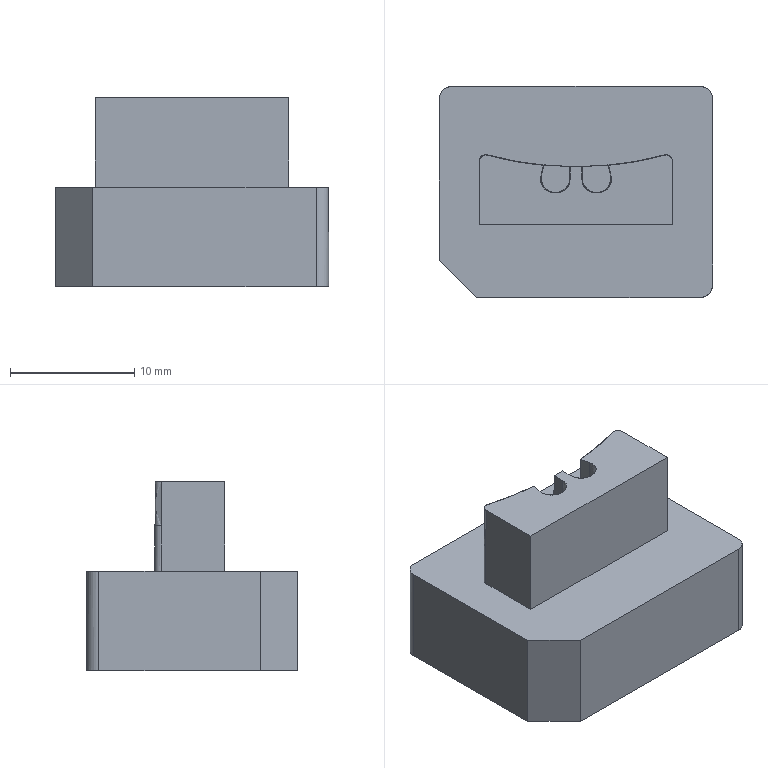NC program | PowerMill | posted by the shop | part box 22 x 17 x 15.232 mm
Lines 5583 to 7135 of 87032:
( TOOL ID   D1C_1_1 )
( TOOL DIA. 1. TIP RAD 0 LENGTH 58.8 )
( Z = -3.721 )
T27 M6
T3
G91 G28 Z0
G0 G90 G54
M08
S22000 M3
X0 Y0 M8
G43 Z9.812 H27
X-2.541 Y2.768
Z.962
G1 Z-.238 F1200
X-2.545 Y2.755 F2000
G3 X-2.454 Y2.605 I.12 J-.03
G1 X-2.412 Y2.594
X-2.315 Y2.533
X-2.171 Y2.359
X-2.144 Y2.292
X-2.123 Y2.051
X-2.29 Y1.327
X-2.323 Y1.086
X-2.299 Y.856
X-2.292 Y.835
X-2.171 Y.636
X-1.995 Y.507
X-1.976 Y.498
X-1.689 Y.44
X-1.447 Y.455
X-1.288 Y.519
X-1.09 Y.713
X-1.027 Y.844
X-.988 Y1.086
X-.99 Y1.915
X-1.45 Y1.92
X-1.459 Y1.085
G2 X-1.607 Y.923 I-.165 J.002
G1 X-1.675 Y.916
G2 X-1.846 Y1.064 I-.016 J.154
G1 X-1.849 Y1.137
X-1.847 Y1.162
X-1.674 Y1.943
X-1.643 Y1.992
X-1.587 Y2.008
X-1.53 Y2.005
X-1.473 Y1.979
X-1.45 Y1.92
X-.99 Y1.915
Y2.051
X-.965 Y2.177
X-.91 Y2.292
X-.724 Y2.458
X-.605 Y2.488
X-2.541 Y2.768 Z-.288
X-2.544 Y2.755
G3 X-2.454 Y2.605 I.12 J-.03
G1 X-2.412 Y2.595
X-2.31 Y2.533
X-2.171 Y2.363
X-2.143 Y2.292
X-2.122 Y2.051
X-2.322 Y1.086
X-2.299 Y.856
X-2.292 Y.834
X-2.171 Y.641
X-1.995 Y.507
X-1.981 Y.501
X-1.976 Y.499
X-1.97 Y.497
X-1.967
X-1.689 Y.441
X-1.447 Y.456
X-1.288 Y.519
X-1.272 Y.535
X-1.091 Y.713
X-1.028 Y.844
X-1.013 Y.929
X-1.007 Y.967
X-.995 Y1.808
X-1.457 Y1.823
X-1.479 Y1.138
G2 X-1.673 Y.971 I-.174 J.006
X-1.824 Y1.178 I.02 J.173
G1 X-1.672 Y1.943
X-1.642 Y1.992
X-1.586 Y2.009
X-1.532 Y2.006
X-1.476 Y1.979
X-1.454 Y1.921
X-1.457 Y1.823
X-.995 Y1.808
X-.991 Y2.051
X-.965 Y2.184
X-.911 Y2.292
X-.724 Y2.459
X-.607 Y2.488
X-2.54 Y2.769 Z-.337
X-2.544 Y2.755
G3 X-2.453 Y2.606 I.12 J-.03
G1 X-2.412 Y2.596
X-2.308 Y2.533
X-2.171 Y2.364
X-2.142 Y2.292
X-2.121 Y2.051
X-2.205 Y1.647
X-1.753 Y1.553
X-1.671 Y1.944
X-1.641 Y1.993
X-1.586 Y2.01
X-1.533 Y2.007
X-1.477 Y1.98
X-1.455 Y1.922
X-1.48 Y1.137
X-1.49 Y1.083
X-1.518 Y1.035
X-1.573 Y.965
G2 X-1.819 Y1.027 I-.109 J.087
G1 X-1.835 Y1.106
X-1.837 Y1.134
X-1.834 Y1.161
X-1.753 Y1.553
X-2.205 Y1.647
X-2.321 Y1.086
X-2.299 Y.856
X-2.292 Y.834
X-2.171 Y.642
X-2.164 Y.635
X-1.999 Y.511
X-1.995 Y.507
X-1.989 Y.505
X-1.972 Y.498
X-1.967 Y.497
X-1.701 Y.443
X-1.689 Y.441
X-1.447 Y.457
X-1.297 Y.516
X-1.283 Y.525
X-1.267 Y.541
X-1.092 Y.713
X-1.029 Y.844
X-1.011 Y.945
X-1.007 Y.966
X-.992 Y2.051
X-.965 Y2.186
X-.912 Y2.292
X-.724 Y2.46
X-.607 Y2.489
X-2.54 Y2.769 Z-.387
X-2.543 Y2.756
G3 X-2.452 Y2.606 I.12 J-.029
G1 X-2.412 Y2.597
X-2.307 Y2.533
X-2.171 Y2.365
X-2.141 Y2.292
X-2.121 Y2.051
X-2.321 Y1.086
X-2.32 Y1.073
X-2.302 Y.887
X-2.3 Y.878
X-2.297 Y.869
X-2.171 Y.643
X-2.162 Y.634
X-2.025 Y.53
X-1.957 Y.494
X-1.715 Y.446
X-1.689 Y.442
X-1.447 Y.457
X-1.297 Y.516
X-1.289 Y.521
X-1.284 Y.524
X-1.279 Y.528
X-1.267 Y.541
X-1.259 Y.548
X-1.093 Y.712
X-1.029 Y.844
X-1.009 Y.953
X-1.007 Y.965
X-.997 Y1.812
X-1.459 Y1.825
X-1.479 Y1.14
G2 X-1.673 Y.971 I-.175 J.005
X-1.825 Y1.18 I.02 J.174
G1 X-1.671 Y1.945
X-1.64 Y1.994
X-1.585 Y2.011
X-1.534 Y2.008
X-1.478 Y1.982
X-1.456 Y1.923
X-1.459 Y1.825
X-.997 Y1.812
X-.994 Y2.051
X-.965 Y2.187
X-.912 Y2.292
X-.724 Y2.461
X-.608 Y2.49
X-2.54 Y2.77 Z-.437
X-2.543 Y2.756
G3 X-2.452 Y2.607 I.12 J-.029
G1 X-2.412 Y2.597
X-2.306 Y2.533
X-2.171 Y2.367
X-2.141 Y2.292
X-2.12 Y2.051
X-2.205 Y1.641
X-1.75 Y1.549
X-1.67 Y1.946
X-1.639 Y1.995
X-1.584 Y2.012
X-1.535 Y2.009
X-1.479 Y1.982
X-1.457 Y1.923
X-1.489 Y1.129
X-1.493 Y1.102
X-1.501 Y1.077
X-1.52 Y1.027
X-1.541 Y.992
X-1.572 Y.964
X-1.608 Y.941
G2 X-1.835 Y1.071 I-.08 J.123
G1 X-1.831 Y1.152
X-1.75 Y1.549
X-2.205 Y1.641
X-2.32 Y1.086
X-2.317 Y1.043
X-2.302 Y.887
X-2.3 Y.878
X-2.297 Y.869
X-2.179 Y.657
X-2.171 Y.644
X-2.156 Y.629
X-2.025 Y.53
X-1.963 Y.497
X-1.957 Y.495
X-1.95 Y.493
X-1.728 Y.448
X-1.689 Y.442
X-1.447 Y.458
X-1.434 Y.462
X-1.308 Y.512
X-1.094 Y.712
X-1.03 Y.844
X-1.009 Y.957
X-1.007 Y.965
X-.995 Y2.051
X-.965 Y2.189
X-.913 Y2.292
X-.724 Y2.462
X-.608 Y2.491
X-2.539 Y2.77 Z-.487
X-2.542 Y2.757
G3 X-2.451 Y2.608 I.12 J-.029
G1 X-2.412 Y2.598
X-2.305 Y2.533
X-2.171 Y2.368
X-2.14 Y2.292
X-2.12 Y2.051
X-2.319 Y1.086
X-2.316 Y1.026
X-2.302 Y.887
X-2.301 Y.878
X-2.297 Y.869
X-2.186 Y.67
X-2.171 Y.645
X-2.151 Y.626
X-2.025 Y.53
X-1.963 Y.497
X-1.957 Y.495
X-1.95 Y.493
X-1.742 Y.451
X-1.689 Y.443
X-1.447 Y.458
X-1.423 Y.467
X-1.316 Y.509
X-1.308 Y.513
X-1.301 Y.518
X-1.261 Y.556
X-1.095 Y.712
X-1.031 Y.844
X-1.008 Y.959
X-1.007 Y.964
X-.999 Y1.814
X-1.461 Y1.827
X-1.481 Y1.142
G2 X-1.675 Y.975 I-.174 J.005
X-1.826 Y1.182 I.02 J.173
G1 X-1.669 Y1.947
X-1.639 Y1.996
X-1.583 Y2.013
X-1.537 Y2.01
X-1.48 Y1.984
X-1.459 Y1.925
X-1.461 Y1.827
X-.999 Y1.814
X-.996 Y2.051
X-.965 Y2.19
X-.914 Y2.292
X-.724 Y2.463
X-.608 Y2.492
X-2.539 Y2.771 Z-.536
X-2.542 Y2.757
G3 X-2.451 Y2.608 I.12 J-.029
G1 X-2.412 Y2.599
X-2.304 Y2.533
X-2.171 Y2.369
X-2.139 Y2.292
X-2.119 Y2.051
X-2.203 Y1.642
X-1.749 Y1.551
X-1.669 Y1.948
X-1.638 Y1.997
X-1.583 Y2.014
X-1.537 Y2.011
X-1.481 Y1.985
X-1.459 Y1.926
X-1.481 Y1.142
X-1.484 Y1.116
X-1.504 Y1.038
X-1.534 Y.982
X-1.586 Y.945
X-1.633 Y.926
G2 X-1.836 Y1.074 I-.056 J.136
G1 X-1.829 Y1.153
X-1.749 Y1.551
X-2.203 Y1.642
X-2.318 Y1.086
X-2.314 Y1.007
X-2.302 Y.887
X-2.301 Y.878
X-2.297 Y.869
X-2.194 Y.684
X-2.174 Y.65
X-2.147 Y.623
X-2.025 Y.53
X-1.963 Y.497
X-1.957 Y.495
X-1.95 Y.493
X-1.756 Y.454
X-1.689 Y.443
X-1.447 Y.459
X-1.41 Y.472
X-1.316 Y.509
X-1.308 Y.513
X-1.301 Y.518
X-1.261 Y.555
X-1.237 Y.578
X-1.096 Y.712
X-1.031 Y.844
X-1.008 Y.964
X-.997 Y2.051
X-.965 Y2.192
X-.914 Y2.292
X-.724 Y2.464
X-.609 Y2.492
X-2.538 Y2.771 Z-.586
X-2.542 Y2.758
G3 X-2.45 Y2.609 I.12 J-.029
G1 X-2.412 Y2.6
X-2.303 Y2.533
X-2.171 Y2.371
X-2.139 Y2.292
X-2.119 Y2.051
X-2.202 Y1.647
X-1.748 Y1.554
X-1.668 Y1.949
X-1.637 Y1.998
X-1.582 Y2.015
X-1.537 Y2.012
X-1.482 Y1.986
X-1.459 Y1.929
X-1.468 Y1.164
X-1.475 Y1.115
X-1.495 Y1.071
X-1.537 Y1.003
X-1.572 Y.965
X-1.62 Y.944
X-1.654 Y.937
G2 X-1.832 Y1.087 I-.031 J.144
G1 X-1.828 Y1.16
X-1.748 Y1.554
X-2.202 Y1.647
X-2.318 Y1.086
X-2.307 Y.935
X-2.303 Y.887
X-2.301 Y.878
X-2.297 Y.869
X-2.194 Y.684
X-2.172 Y.648
X-2.142 Y.619
X-2.025 Y.529
X-1.966 Y.499
X-1.955 Y.494
X-1.77 Y.457
X-1.689 Y.443
X-1.459 Y.459
X-1.438 Y.465
X-1.242 Y.573
X-1.237 Y.578
X-1.103 Y.704
X-1.098 Y.711
X-1.093 Y.718
X-1.032 Y.844
X-1.008 Y.964
X-.997 Y2.051
X-.965 Y2.193
X-.915 Y2.292
X-.724 Y2.465
X-.609 Y2.493
X-2.538 Y2.772 Z-.636
X-2.541 Y2.758
G3 X-2.449 Y2.609 I.12 J-.028
G1 X-2.412 Y2.601
X-2.302 Y2.533
X-2.171 Y2.372
X-2.138 Y2.292
X-2.118 Y2.051
X-2.201 Y1.648
X-1.748 Y1.556
X-1.667 Y1.95
X-1.637 Y1.999
X-1.581 Y2.016
X-1.538 Y2.013
X-1.482 Y1.987
X-1.46 Y1.929
X-1.471 Y1.155
X-1.479 Y1.107
X-1.5 Y1.063
X-1.543 Y.998
X-1.572 Y.968
X-1.609 Y.948
X-1.64 Y.937
G2 X-1.833 Y1.086 I-.046 J.14
G1 X-1.828 Y1.161
X-1.748 Y1.556
X-2.201 Y1.648
X-2.317 Y1.086
X-2.304 Y.905
X-2.303 Y.887
X-2.301 Y.878
X-2.297 Y.869
X-2.198 Y.692
X-2.173 Y.649
X-2.137 Y.615
X-2.025 Y.529
X-1.974 Y.503
X-1.952 Y.493
X-1.784 Y.459
X-1.689 Y.444
X-1.459 Y.46
X-1.438 Y.466
X-1.24 Y.575
X-1.108 Y.7
X-1.097 Y.712
X-1.033 Y.844
X-1.009 Y.964
X-.998 Y2.051
X-.965 Y2.195
X-.916 Y2.292
X-.724 Y2.466
X-.609 Y2.494
X-2.537 Y2.772 Z-.686
X-2.541 Y2.759
G3 X-2.448 Y2.61 I.12 J-.028
G1 X-2.412 Y2.602
X-2.301 Y2.533
X-2.171 Y2.374
X-2.137 Y2.292
X-2.117 Y2.051
X-2.2 Y1.649
X-1.747 Y1.556
X-1.667 Y1.95
X-1.636 Y1.999
X-1.581 Y2.016
X-1.538 Y2.014
X-1.483 Y1.988
X-1.46 Y1.93
X-1.47 Y1.156
X-1.478 Y1.107
X-1.5 Y1.062
X-1.546 Y.996
X-1.573 Y.967
X-1.609 Y.948
X-1.64 Y.937
G2 X-1.834 Y1.088 I-.048 J.139
G1 X-1.828 Y1.162
X-1.747 Y1.556
X-2.2 Y1.649
X-2.316 Y1.086
X-2.302 Y.888
X-2.301 Y.878
X-2.297 Y.868
X-2.204 Y.702
X-2.174 Y.652
X-2.132 Y.611
X-2.025 Y.529
X-1.983 Y.507
X-1.95 Y.493
X-1.798 Y.462
X-1.689 Y.444
X-1.459 Y.46
X-1.438 Y.466
X-1.238 Y.577
X-1.114 Y.694
X-1.098 Y.712
X-1.033 Y.844
X-1.009 Y.964
X-.998 Y2.051
X-.965 Y2.196
X-.917 Y2.292
X-.724 Y2.467
X-.61 Y2.495
X-2.537 Y2.773 Z-.735
X-2.54 Y2.759
G3 X-2.448 Y2.611 I.121 J-.028
G1 X-2.412 Y2.602
X-2.3 Y2.533
X-2.171 Y2.375
X-2.136 Y2.292
X-2.117 Y2.051
X-2.199 Y1.651
X-1.747 Y1.558
X-1.666 Y1.951
X-1.635 Y2.
X-1.58 Y2.017
X-1.539 Y2.015
X-1.483 Y1.989
X-1.461 Y1.931
X-1.469 Y1.157
X-1.482 Y1.094
X-1.517 Y1.041
X-1.583 Y.973
G2 X-1.835 Y1.086 I-.106 J.103
G1 X-1.829 Y1.164
X-1.747 Y1.558
X-2.199 Y1.651
X-2.316 Y1.086
X-2.296 Y.874
X-2.294 Y.865
X-2.29 Y.856
X-2.208 Y.708
X-2.175 Y.654
X-2.13 Y.609
X-2.025 Y.529
X-2.004 Y.518
X-1.947 Y.492
X-1.812 Y.465
X-1.689 Y.445
X-1.459 Y.461
X-1.438 Y.467
X-1.236 Y.579
X-1.121 Y.688
X-1.099 Y.712
X-1.034 Y.844
X-1.01 Y.964
X-.999 Y2.051
X-.965 Y2.198
X-.917 Y2.292
X-.724 Y2.468
X-.61 Y2.496
X-2.537 Y2.773 Z-.785
X-2.54 Y2.76
G3 X-2.447 Y2.611 I.121 J-.028
G1 X-2.412 Y2.603
X-2.299 Y2.533
X-2.171 Y2.376
X-2.136 Y2.292
X-2.116 Y2.051
X-2.315 Y1.086
X-2.295 Y.873
X-2.293 Y.863
X-2.289 Y.854
X-2.213 Y.718
X-2.176 Y.657
X-2.125 Y.606
X-2.025 Y.529
X-2.011 Y.522
X-1.945 Y.492
X-1.826 Y.468
X-1.689 Y.445
X-1.459 Y.462
X-1.438 Y.468
X-1.233 Y.581
X-1.128 Y.681
X-1.099 Y.712
X-1.035 Y.844
X-1.009 Y1.028
X-1.004 Y1.53
X-1.466 Y1.538
X-1.473 Y1.144
G2 X-1.67 Y.971 I-.177 J.003
X-1.824 Y1.183 I.019 J.176
G1 X-1.665 Y1.952
X-1.635 Y2.001
X-1.58 Y2.018
X-1.538 Y2.016
X-1.482 Y1.989
X-1.46 Y1.932
X-1.466 Y1.538
X-1.004 Y1.53
X-.999 Y1.989
Y2.051
X-.998 Y2.055
X-.965 Y2.198
X-.92 Y2.287
X-.918 Y2.292
X-.724 Y2.469
X-.61 Y2.497
X-2.536 Y2.774 Z-.835
X-2.539 Y2.76
G3 X-2.446 Y2.612 I.121 J-.028
G1 X-2.412 Y2.604
X-2.298 Y2.533
X-2.171 Y2.378
X-2.135 Y2.292
X-2.116 Y2.051
X-2.198 Y1.651
X-1.746 Y1.558
X-1.665 Y1.953
X-1.634 Y2.002
X-1.579 Y2.019
X-1.537 Y2.017
X-1.481 Y1.99
X-1.459 Y1.932
X-1.475 Y1.164
X-1.49 Y1.096
X-1.529 Y1.039
X-1.581 Y.986
G2 X-1.832 Y1.1 I-.104 J.104
G1 X-1.827 Y1.163
X-1.746 Y1.558
X-2.198 Y1.651
X-2.315 Y1.086
X-2.294 Y.871
X-2.292 Y.861
X-2.288 Y.853
X-2.219 Y.728
X-2.171 Y.651
X-2.102 Y.586
X-2.026 Y.53
X-1.942 Y.491
X-1.841 Y.471
X-1.689 Y.446
X-1.459 Y.462
X-1.438 Y.468
X-1.231 Y.583
X-1.134 Y.675
X-1.1 Y.712
X-1.036 Y.844
X-1.009 Y1.032
X-1. Y1.928
Y2.051
X-.996 Y2.06
X-.965 Y2.198
X-.922 Y2.283
X-.919 Y2.292
X-.724 Y2.47
X-.609 Y2.498
X-2.536 Y2.774 Z-.885
X-2.539 Y2.761
G3 X-2.446 Y2.612 I.121 J-.028
G1 X-2.412 Y2.605
X-2.297 Y2.533
X-2.171 Y2.379
X-2.134 Y2.292
X-2.116 Y2.051
X-2.314 Y1.086
X-2.293 Y.869
X-2.291 Y.86
X-2.287 Y.851
X-2.23 Y.746
X-2.163 Y.646
X-1.943 Y.495
X-1.935 Y.491
X-1.926 Y.488
X-1.859 Y.474
X-1.689 Y.446
X-1.459 Y.463
X-1.438 Y.469
X-1.229 Y.585
X-1.141 Y.669
X-1.101 Y.712
X-1.036 Y.844
X-1.009 Y1.036
X-1.004 Y1.506
X-1.465 Y1.514
X-1.472 Y1.094
G2 X-1.657 Y.945 I-.155 J.003
G1 X-1.712 Y.956
G2 X-1.832 Y1.137 I.03 J.151
G1 X-1.664 Y1.954
X-1.634 Y2.003
X-1.579 Y2.02
X-1.536 Y2.017
X-1.48 Y1.991
X-1.458 Y1.934
X-1.465 Y1.514
X-1.004 Y1.506
X-1. Y1.867
Y2.051
X-.995 Y2.065
X-.965 Y2.198
X-.924 Y2.278
X-.919 Y2.292
X-.724 Y2.471
X-.609 Y2.499
X-2.535 Y2.775 Z-.934
X-2.538 Y2.761
G3 X-2.445 Y2.613 I.121 J-.027
G1 X-2.412 Y2.606
X-2.296 Y2.533
X-2.171 Y2.38
X-2.133 Y2.292
X-2.115 Y2.051
X-2.314 Y1.086
X-2.292 Y.867
X-2.29 Y.858
X-2.286 Y.849
X-2.229 Y.745
X-2.163 Y.647
X-1.942 Y.495
X-1.933 Y.49
X-1.924 Y.487
X-1.877 Y.478
X-1.689 Y.447
X-1.459 Y.463
X-1.438 Y.47
X-1.227 Y.588
X-1.147 Y.663
X-1.102 Y.712
X-1.037 Y.844
X-1.009 Y1.04
X-1.004 Y1.51
X-1.467 Y1.515
X-1.471 Y1.095
G2 X-1.657 Y.945 I-.155 J.002
G1 X-1.712 Y.956
G2 X-1.831 Y1.137 I.031 J.15
G1 X-1.664 Y1.955
X-1.633 Y2.004
X-1.578 Y2.02
X-1.54 Y2.018
X-1.485 Y1.992
X-1.462 Y1.935
X-1.467 Y1.515
X-1.004 Y1.51
X-1.001 Y1.807
Y2.051
X-.994 Y2.071
X-.965 Y2.198
X-.926 Y2.274
X-.92 Y2.292
X-.724 Y2.472
X-.609 Y2.5
X-2.535 Y2.775 Z-.984
X-2.538 Y2.762
G3 X-2.444 Y2.614 I.121 J-.027
G1 X-2.412 Y2.607
X-2.295 Y2.533
X-2.171 Y2.382
X-2.133 Y2.292
X-2.115 Y2.051
X-2.313 Y1.086
X-2.291 Y.866
X-2.289 Y.856
X-2.285 Y.847
X-2.228 Y.745
X-2.163 Y.648
X-1.939 Y.494
X-1.929 Y.488
X-1.897 Y.482
X-1.689 Y.447
X-1.459 Y.464
X-1.438 Y.47
X-1.224 Y.59
X-1.154 Y.656
X-1.102 Y.712
X-1.038 Y.844
X-1.009 Y1.044
X-1.002 Y1.747
X-1.001 Y1.925
X-1.463 Y1.935
X-1.48 Y1.126
G2 X-1.656 Y.969 I-.161 J.003
X-1.8 Y1.157 I.015 J.16
G1 X-1.664 Y1.953
X-1.634 Y2.003
X-1.578 Y2.021
X-1.541 Y2.019
X-1.485 Y1.993
X-1.463 Y1.935
X-1.001 Y1.925
Y2.051
X-.993 Y2.076
X-.965 Y2.198
X-.928 Y2.27
X-.921 Y2.292
X-.724 Y2.473
X-.609 Y2.501
X-2.534 Y2.775 Z-1.034
X-2.537 Y2.762
G3 X-2.444 Y2.614 I.121 J-.027
G1 X-2.412 Y2.607
X-2.294 Y2.533
X-2.171 Y2.383
X-2.132 Y2.292
X-2.114 Y2.051
X-2.313 Y1.086
X-2.29 Y.864
X-2.288 Y.855
X-2.285 Y.846
X-2.228 Y.745
X-2.163 Y.649
X-1.939 Y.494
X-1.928 Y.489
X-1.922 Y.487
X-1.916 Y.486
X-1.689 Y.448
X-1.459 Y.465
X-1.438 Y.471
X-1.222 Y.592
X-1.16 Y.65
X-1.103 Y.712
X-1.038 Y.844
X-1.009 Y1.048
X-1.002 Y1.688
Y1.928
X-1.463 Y1.936
X-1.477 Y1.129
G2 X-1.655 Y.97 I-.163 J.003
X-1.8 Y1.159 I.015 J.162
G1 X-1.663 Y1.954
X-1.633 Y2.004
X-1.577 Y2.022
X-1.541 Y2.02
X-1.485 Y1.994
X-1.463 Y1.936
X-1.002 Y1.928
Y2.051
X-.97 Y2.174
X-.922 Y2.292
X-.724 Y2.473
X-.608 Y2.502
X-2.534 Y2.776 Z-1.084
X-2.537 Y2.763
G3 X-2.443 Y2.615 I.121 J-.027
G1 X-2.412 Y2.608
X-2.293 Y2.533
X-2.171 Y2.384
X-2.131 Y2.292
X-2.114 Y2.051
X-2.312 Y1.086
X-2.289 Y.862
X-2.287 Y.853
X-2.284 Y.844
X-2.227 Y.744
X-2.163 Y.65
X-1.939 Y.495
X-1.919 Y.487
X-1.689 Y.448
X-1.459 Y.465
X-1.438 Y.472
X-1.22 Y.594
X-1.167 Y.644
X-1.104 Y.712
X-1.039 Y.844
X-1.008 Y1.052
X-1.003 Y1.629
X-1.002 Y1.919
X-1.464 Y1.935
X-1.492 Y1.147
G2 X-1.675 Y.99 I-.164 J.006
X-1.816 Y1.185 I.019 J.163
G1 X-1.662 Y1.957
X-1.632 Y2.006
X-1.576 Y2.023
X-1.541 Y2.021
X-1.485 Y1.994
X-1.464 Y1.935
X-1.002 Y1.919
Y2.051
X-.97 Y2.174
X-.922 Y2.292
X-.724 Y2.474
X-.608 Y2.502
X-2.533 Y2.776 Z-1.133
X-2.536 Y2.763
G3 X-2.442 Y2.615 I.121 J-.027
G1 X-2.412 Y2.609
X-2.292 Y2.533
X-2.171 Y2.386
X-2.131 Y2.292
X-2.113 Y2.051
X-2.312 Y1.086
X-2.288 Y.86
X-2.286 Y.851
X-2.283 Y.842
X-2.227 Y.744
X-2.163 Y.651
X-1.939 Y.496
X-1.919 Y.487
X-1.689 Y.449
X-1.459 Y.466
X-1.438 Y.472
X-1.217 Y.596
X-1.174 Y.637
X-1.105 Y.712
X-1.04 Y.844
X-1.008 Y1.055
X-1.003 Y1.571
Y1.92
X-1.464 Y1.936
X-1.492 Y1.148
G2 X-1.674 Y.991 I-.164 J.006
X-1.816 Y1.185 I.019 J.163
G1 X-1.662 Y1.957
X-1.631 Y2.007
X-1.576 Y2.024
X-1.542 Y2.022
X-1.485 Y1.995
X-1.464 Y1.936
X-1.003 Y1.92
Y2.051
X-.969 Y2.173
X-.923 Y2.292
X-.724 Y2.475
X-.609 Y2.505
X-2.533 Y2.777 Z-1.183
X-2.536 Y2.763
G3 X-2.442 Y2.616 I.121 J-.027
G1 X-2.412 Y2.609
X-2.291 Y2.533
X-2.171 Y2.387
X-2.13 Y2.292
X-2.113 Y2.051
X-2.311 Y1.086
X-2.287 Y.858
X-2.286 Y.849
X-2.282 Y.841
X-2.227 Y.743
X-2.163 Y.652
X-1.939 Y.496
X-1.919 Y.488
X-1.689 Y.449
X-1.458 Y.467
X-1.438 Y.473
X-1.215 Y.598
X-1.18 Y.631
X-1.105 Y.711
X-1.04 Y.844
X-1.008 Y1.059
X-1.004 Y1.513
X-1.003 Y1.922
X-1.464 Y1.937
X-1.491 Y1.149
G2 X-1.674 Y.991 I-.164 J.006
X-1.816 Y1.186 I.019 J.163
G1 X-1.661 Y1.958
X-1.631 Y2.007
X-1.575 Y2.024
X-1.542 Y2.022
X-1.486 Y1.996
X-1.464 Y1.937
X-1.003 Y1.922
Y2.051
X-.969 Y2.173
X-.924 Y2.292
X-.724 Y2.475
X-.61 Y2.506
X-2.533 Y2.777 Z-1.233
X-2.536 Y2.764
G3 X-2.441 Y2.616 I.121 J-.027
G1 X-2.412 Y2.61
X-2.29 Y2.533
X-2.171 Y2.388
X-2.129 Y2.292
X-2.112 Y2.051
X-2.311 Y1.086
X-2.286 Y.856
X-2.284 Y.844
X-2.272 Y.823
X-2.177 Y.668
X-2.163 Y.653
X-1.939 Y.497
X-1.919 Y.489
X-1.689 Y.449
X-1.458 Y.467
X-1.438 Y.474
X-1.213 Y.6
X-1.189 Y.623
X-1.106 Y.712
X-1.041 Y.844
X-1.008 Y1.063
X-1.004 Y1.456
Y1.923
X-1.465 Y1.938
X-1.491 Y1.148
G2 X-1.673 Y.992 I-.163 J.005
X-1.814 Y1.185 I.019 J.162
G1 X-1.661 Y1.959
X-1.63 Y2.008
X-1.575 Y2.025
X-1.542 Y2.023
X-1.486 Y1.997
X-1.465 Y1.938
X-1.004 Y1.923
X-1.003 Y2.051
X-.969 Y2.173
X-.924 Y2.292
X-.724 Y2.476
X-.61 Y2.508
X-2.532 Y2.778 Z-1.283
X-2.535 Y2.764
G3 X-2.441 Y2.617 I.121 J-.026
G1 X-2.412 Y2.611
X-2.289 Y2.533
X-2.171 Y2.39
X-2.129 Y2.292
X-2.112 Y2.051
X-2.197 Y1.637
X-1.746 Y1.544
X-1.66 Y1.96
X-1.629 Y2.009
X-1.574 Y2.026
X-1.543 Y2.024
X-1.487 Y1.998
X-1.465 Y1.94
X-1.481 Y1.093
G2 X-1.634 Y.948 I-.147 J.003
G1 X-1.693 Y.951
G2 X-1.832 Y1.127 I.006 J.147
G1 X-1.746 Y1.544
X-2.197 Y1.637
X-2.31 Y1.086
X-2.286 Y.856
X-2.279 Y.835
X-2.177 Y.669
X-2.163 Y.654
X-1.939 Y.498
X-1.919 Y.489
X-1.689 Y.45
X-1.458 Y.468
X-1.438 Y.474
X-1.212 Y.601
X-1.197 Y.615
X-1.106 Y.712
X-1.042 Y.844
X-1.008 Y1.066
X-1.005 Y1.399
X-1.004 Y2.051
X-.969 Y2.173
X-.925 Y2.292
X-.724 Y2.477
X-.61 Y2.509
X-2.532 Y2.778 Z-1.332
X-2.535 Y2.765
G3 X-2.44 Y2.617 I.121 J-.026
G1 X-2.412 Y2.611
X-2.288 Y2.533
X-2.171 Y2.391
X-2.128 Y2.292
X-2.111 Y2.051
X-2.196 Y1.637
X-1.745 Y1.544
X-1.659 Y1.961
X-1.629 Y2.01
X-1.574 Y2.027
X-1.543 Y2.025
X-1.487 Y1.999
X-1.466 Y1.941
X-1.48 Y1.093
G2 X-1.633 Y.949 I-.147 J.003
G1 X-1.693 Y.951
G2 X-1.831 Y1.128 I.005 J.147
G1 X-1.745 Y1.544
X-2.196 Y1.637
X-2.31 Y1.086
X-2.285 Y.856
X-2.278 Y.835
X-2.177 Y.67
X-2.163 Y.655
X-1.939 Y.498
X-1.919 Y.49
X-1.689 Y.45
X-1.458 Y.469
X-1.438 Y.475
X-1.215 Y.6
X-1.209 Y.604
X-1.204 Y.608
X-1.107 Y.713
X-1.042 Y.844
X-1.008 Y1.07
X-1.005 Y1.342
X-1.004 Y2.051
X-.969 Y2.172
X-.926 Y2.292
X-.724 Y2.477
X-.61 Y2.51
X-2.531 Y2.779 Z-1.382
X-2.534 Y2.765
G3 X-2.44 Y2.618 I.121 J-.026
G1 X-2.412 Y2.612
X-2.287 Y2.533
X-2.171 Y2.392
X-2.127 Y2.292
X-2.111 Y2.051
X-2.309 Y1.086
X-2.284 Y.855
X-2.277 Y.835
X-2.177 Y.671
X-2.163 Y.656
X-1.939 Y.499
X-1.919 Y.491
X-1.689 Y.451
X-1.458 Y.469
X-1.438 Y.475
X-1.21 Y.603
X-1.107 Y.713
X-1.043 Y.844
X-1.008 Y1.073
X-1.006 Y1.286
X-1.005 Y1.828
X-1.468 Y1.836
X-1.48 Y1.094
G2 X-1.643 Y.95 I-.147 J.002
G1 X-1.696 Y.956
G2 X-1.818 Y1.12 I.015 J.139
G1 X-1.659 Y1.961
X-1.629 Y2.01
X-1.573 Y2.028
X-1.543 Y2.026
X-1.488 Y2.
X-1.466 Y1.942
X-1.468 Y1.836
X-1.005 Y1.828
Y2.051
X-.969 Y2.172
X-.927 Y2.292
X-.724 Y2.478
X-.61 Y2.512
X-2.531 Y2.779 Z-1.432
X-2.534 Y2.766
G3 X-2.439 Y2.618 I.121 J-.026
G1 X-2.412 Y2.613
X-2.286 Y2.533
X-2.171 Y2.394
X-2.127 Y2.292
X-2.11 Y2.051
X-2.309 Y1.086
X-2.283 Y.855
X-2.276 Y.835
X-2.177 Y.671
X-2.163 Y.657
X-1.939 Y.5
X-1.919 Y.491
X-1.689 Y.451
X-1.458 Y.47
X-1.438 Y.476
X-1.211 Y.603
X-1.107 Y.714
X-1.044 Y.844
X-1.008 Y1.077
X-1.006 Y1.231
X-1.005 Y1.936
X-1.466 Y1.943
X-1.479 Y1.094
G2 X-1.642 Y.95 I-.147 J.002
G1 X-1.696 Y.956
G2 X-1.818 Y1.121 I.015 J.139
G1 X-1.659 Y1.961
X-1.628 Y2.011
X-1.573 Y2.028
X-1.544 Y2.027
X-1.488 Y2.
X-1.466 Y1.943
X-1.005 Y1.936
Y2.051
X-.982 Y2.123
X-.964 Y2.198
X-.942 Y2.243
X-.927 Y2.292
X-.724 Y2.479
X-.61 Y2.513
X-2.531 Y2.779 Z-1.482
X-2.534 Y2.766
G3 X-2.439 Y2.619 I.121 J-.026
G1 X-2.412 Y2.613
X-2.285 Y2.533
X-2.171 Y2.395
X-2.126 Y2.292
X-2.11 Y2.051
X-2.308 Y1.086
X-2.283 Y.855
X-2.276 Y.835
X-2.177 Y.672
X-2.163 Y.657
X-1.939 Y.5
X-1.919 Y.492
X-1.689 Y.452
X-1.458 Y.47
X-1.438 Y.477
X-1.212 Y.603
X-1.108 Y.714
X-1.044 Y.844
X-1.008 Y1.08
X-1.007 Y1.176
X-1.006 Y1.937
X-1.467 Y1.944
X-1.479 Y1.095
G2 X-1.641 Y.951 I-.147 J.002
G1 X-1.696 Y.956
G2 X-1.819 Y1.122 I.014 J.139
G1 X-1.658 Y1.962
X-1.628 Y2.012
X-1.572 Y2.029
X-1.544 Y2.027
X-1.489 Y2.001
X-1.467 Y1.944
X-1.006 Y1.937
Y2.051
X-.982 Y2.123
X-.964 Y2.197
X-.942 Y2.243
X-.928 Y2.292
X-.724 Y2.479
X-.61 Y2.514
X-2.53 Y2.78 Z-1.531
X-2.533 Y2.766
G3 X-2.438 Y2.619 I.121 J-.026
G1 X-2.412 Y2.614
X-2.284 Y2.533
X-2.171 Y2.396
X-2.125 Y2.292
X-2.109 Y2.051
X-2.308 Y1.086
X-2.282 Y.855
X-2.275 Y.835
X-2.177 Y.673
X-2.163 Y.658
X-1.939 Y.501
X-1.919 Y.493
X-1.689 Y.452
X-1.458 Y.471
X-1.438 Y.477
X-1.213 Y.603
X-1.108 Y.715
X-1.045 Y.844
X-1.008 Y1.083
X-1.007 Y1.121
X-1.006 Y1.926
X-1.467 Y1.943
X-1.497 Y1.145
G2 X-1.672 Y.995 I-.157 J.006
X-1.809 Y1.181 I.018 J.156
G1 X-1.658 Y1.962
X-1.627 Y2.012
X-1.572 Y2.03
X-1.545 Y2.028
X-1.488 Y2.001
X-1.467 Y1.943
X-1.006 Y1.926
Y2.051
X-.977 Y2.141
X-.969 Y2.185
X-.95 Y2.225
X-.929 Y2.292
X-.724 Y2.48
X-.61 Y2.515
X-2.53 Y2.78 Z-1.581
X-2.533 Y2.767
G3 X-2.438 Y2.62 I.121 J-.026
G1 X-2.412 Y2.614
X-2.283 Y2.533
X-2.171 Y2.398
X-2.125 Y2.292
X-2.109 Y2.051
X-2.307 Y1.086
X-2.281 Y.855
X-2.274 Y.835
X-2.177 Y.674
X-2.163 Y.659
X-1.939 Y.502
X-1.919 Y.493
X-1.689 Y.452
X-1.458 Y.472
X-1.438 Y.478
X-1.214 Y.603
X-1.109 Y.715
X-1.045 Y.844
X-1.008 Y1.086
X-1.007 Y1.94
X-1.467 Y1.946
X-1.478 Y1.096
G2 X-1.64 Y.952 I-.147 J.002
G1 X-1.696 Y.957
G2 X-1.819 Y1.123 I.014 J.139
G1 X-1.657 Y1.963
X-1.627 Y2.013
X-1.571 Y2.031
X-1.545 Y2.029
X-1.49 Y2.003
X-1.467 Y1.946
X-1.007 Y1.94
Y2.051
X-.976 Y2.147
X-.968 Y2.186
X-.952 Y2.222
X-.929 Y2.292
X-.724 Y2.481
X-.609 Y2.516
X-2.53 Y2.781 Z-1.631
X-2.532 Y2.767
G3 X-2.437 Y2.62 I.121 J-.026
G1 X-2.412 Y2.615
X-2.282 Y2.533
X-2.171 Y2.399
X-2.124 Y2.292
X-2.109 Y2.051
X-2.195 Y1.632
X-1.738 Y1.543
X-1.657 Y1.963
X-1.627 Y2.014
X-1.571 Y2.032
X-1.545 Y2.03
X-1.49 Y2.004
X-1.468 Y1.947
X-1.477 Y1.097
G2 X-1.639 Y.952 I-.147 J.002
G1 X-1.697 Y.958
G2 X-1.82 Y1.123 I.014 J.139
G1 X-1.738 Y1.543
X-2.195 Y1.632
X-2.307 Y1.086
X-2.28 Y.855
X-2.274 Y.835
X-2.177 Y.675
X-2.163 Y.66
X-1.939 Y.503
X-1.919 Y.494
X-1.689 Y.453
X-1.458 Y.472
X-1.438 Y.478
X-1.215 Y.603
X-1.109 Y.716
X-1.046 Y.844
X-1.008 Y1.086
X-1.007 Y2.051
X-.974 Y2.154
X-.968 Y2.187
X-.954 Y2.218
X-.93 Y2.292
X-.724 Y2.481
X-.609 Y2.517
X-2.529 Y2.781 Z-1.681
X-2.532 Y2.768
G3 X-2.437 Y2.621 I.121 J-.026
G1 X-2.412 Y2.616
X-2.281 Y2.533
X-2.171 Y2.4
X-2.123 Y2.292
X-2.108 Y2.051
X-2.194 Y1.633
X-1.738 Y1.544
X-1.656 Y1.963
X-1.626 Y2.014
X-1.57 Y2.032
X-1.546 Y2.031
X-1.49 Y2.005
X-1.468 Y1.948
X-1.477 Y1.097
G2 X-1.638 Y.952 I-.147 J.001
G1 X-1.697 Y.958
G2 X-1.82 Y1.124 I.014 J.139
G1 X-1.738 Y1.544
X-2.194 Y1.633
X-2.306 Y1.086
X-2.28 Y.855
X-2.273 Y.835
X-2.177 Y.676
X-2.163 Y.661
X-1.939 Y.503
X-1.919 Y.495
X-1.689 Y.453
X-1.458 Y.473
X-1.438 Y.479
X-1.216 Y.603
X-1.109 Y.716
X-1.047 Y.844
X-1.009 Y1.086
X-1.008 Y2.051
X-.972 Y2.161
X-.964 Y2.197
X-.955 Y2.214
X-.931 Y2.292
X-.724 Y2.482
X-.609 Y2.518
X-2.529 Y2.782 Z-1.73
X-2.532 Y2.768
G3 X-2.436 Y2.621 I.121 J-.026
G1 X-2.412 Y2.616
X-2.28 Y2.533
X-2.171 Y2.402
X-2.123 Y2.292
X-2.108 Y2.051
X-2.193 Y1.633
X-1.738 Y1.544
X-1.656 Y1.964
X-1.626 Y2.015
X-1.57 Y2.033
X-1.546 Y2.032
X-1.491 Y2.006
X-1.469 Y1.949
X-1.476 Y1.098
G2 X-1.638 Y.953 I-.147 J.001
G1 X-1.697 Y.959
G2 X-1.82 Y1.125 I.014 J.139
G1 X-1.738 Y1.544
X-2.193 Y1.633
X-2.306 Y1.086
X-2.279 Y.855
X-2.272 Y.835
X-2.177 Y.677
X-2.163 Y.662
X-1.939 Y.504
X-1.919 Y.495
X-1.689 Y.454
X-1.458 Y.474
X-1.438 Y.48
X-1.217 Y.603
X-1.11 Y.717
X-1.047 Y.844
X-1.009 Y1.086
X-1.008 Y2.051
X-.971 Y2.168
X-.964 Y2.197
X-.957 Y2.211
X-.932 Y2.292
X-.724 Y2.483
X-.609 Y2.519
X-2.528 Y2.782 Z-1.78
X-2.531 Y2.769
G3 X-2.436 Y2.622 I.121 J-.026
G1 X-2.412 Y2.617
X-2.279 Y2.533
X-2.171 Y2.403
X-2.122 Y2.292
X-2.107 Y2.051
X-2.193 Y1.634
X-1.738 Y1.545
X-1.655 Y1.964
X-1.626 Y2.016
X-1.569 Y2.034
X-1.547 Y2.033
X-1.491 Y2.007
X-1.469 Y1.95
X-1.475 Y1.099
G2 X-1.637 Y.953 I-.147 J.001
G1 X-1.697 Y.959
G2 X-1.821 Y1.125 I.014 J.139
G1 X-1.738 Y1.545
X-2.193 Y1.634
X-2.305 Y1.086
X-2.278 Y.855
X-2.271 Y.835
X-2.177 Y.678
X-2.163 Y.663
X-1.939 Y.505
X-1.919 Y.496
X-1.689 Y.454
X-1.458 Y.474
X-1.438 Y.48
X-1.218 Y.603
X-1.11 Y.717
X-1.048 Y.844
X-1.009 Y1.086
Y2.051
X-.969 Y2.176
X-.964 Y2.197
X-.959 Y2.207
X-.932 Y2.292
X-.724 Y2.483
X-.609 Y2.52
X-2.528 Y2.782 Z-1.83
X-2.531 Y2.769
G3 X-2.435 Y2.622 I.121 J-.026
G1 X-2.412 Y2.618
X-2.278 Y2.533
X-2.171 Y2.404
X-2.121 Y2.292
X-2.107 Y2.051
X-2.305 Y1.086
X-2.277 Y.855
X-2.271 Y.835
X-2.177 Y.679
X-2.163 Y.664
X-1.939 Y.505
X-1.919 Y.497
X-1.689 Y.455
X-1.458 Y.475
X-1.438 Y.481
X-1.219 Y.603
X-1.111 Y.718
X-1.048 Y.844
X-1.01 Y1.086
X-1.009 Y1.832
X-1.472 Y1.842
X-1.489 Y1.094
G2 X-1.633 Y.957 I-.14 J.003
G1 X-1.689 Y.959
G2 X-1.821 Y1.126 I.005 J.14
G1 X-1.655 Y1.964
X-1.626 Y2.016
X-1.569 Y2.035
X-1.547 Y2.033
X-1.491 Y2.007
X-1.47 Y1.949
X-1.472 Y1.842
X-1.009 Y1.832
Y2.051
X-.967 Y2.183
X-.964 Y2.197
X-.961 Y2.204
X-.933 Y2.292
X-.724 Y2.484
X-.61 Y2.521
X-2.528 Y2.783 Z-1.88
X-2.53 Y2.769
G3 X-2.435 Y2.623 I.121 J-.026
G1 X-2.412 Y2.618
X-2.277 Y2.533
X-2.171 Y2.406
X-2.121 Y2.292
X-2.106 Y2.051
X-2.304 Y1.086
X-2.277 Y.855
X-2.27 Y.835
X-2.177 Y.68
X-2.163 Y.665
X-1.939 Y.506
X-1.919 Y.497
X-1.689 Y.455
X-1.458 Y.475
X-1.438 Y.482
X-1.22 Y.603
X-1.111 Y.718
X-1.049 Y.844
X-1.01 Y1.086
Y1.931
X-1.47 Y1.949
X-1.502 Y1.143
G2 X-1.67 Y.998 I-.151 J.006
X-1.802 Y1.177 I.017 J.151
G1 X-1.654 Y1.965
X-1.625 Y2.017